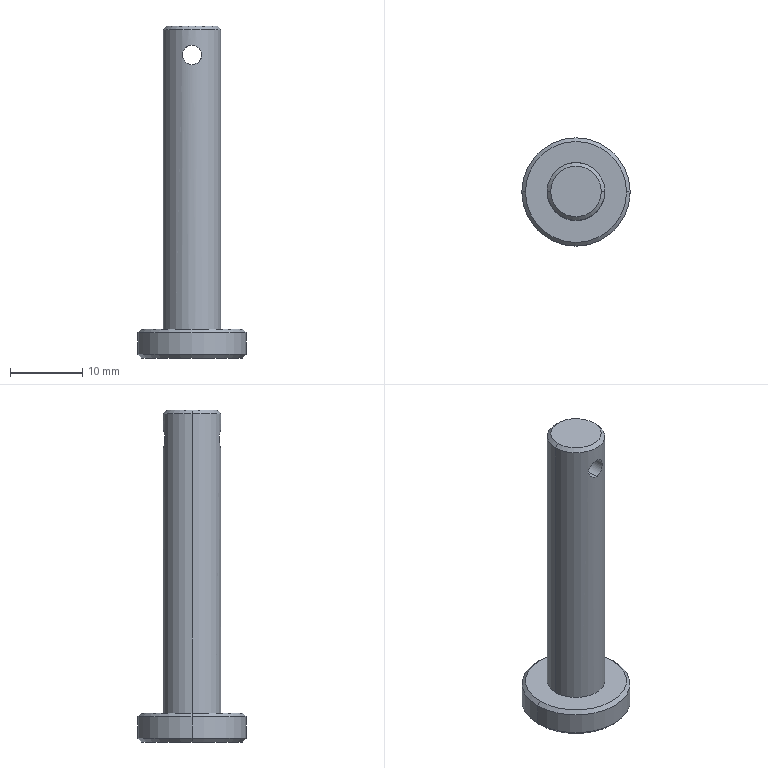Part | SolidWorks | features ICE 2, Chamfer 1, Extrusion 1 | 1 solid | 15 faces | box 15 x 15 x 46 mm | volume 2758 mm3 | cone 6 | cylinder 6 | plane 3 | commonest cylinder face diameters 2.7 x2 8 x2 15 x2
STEP:
#1=CARTESIAN_POINT('',(3.5,0.,42.));
#2=VERTEX_POINT('',#1);
#3=CARTESIAN_POINT('',(-3.5,0.,42.));
#4=VERTEX_POINT('',#3);
#5=CARTESIAN_POINT('',(0.,0.,42.));
#6=DIRECTION('',(0.,0.,1.));
#7=DIRECTION('',(1.,0.,0.));
#8=AXIS2_PLACEMENT_3D('',#5,#6,#7);
#9=CIRCLE('',#8,3.5);
#10=EDGE_CURVE('',#2,#4,#9,.T.);
#11=ORIENTED_EDGE('',*,*,#10,.F.);
#12=CARTESIAN_POINT('',(4.,0.,41.5));
#13=VERTEX_POINT('',#12);
#14=CARTESIAN_POINT('',(3.5,0.,42.));
#15=DIRECTION('',(0.7071,0.,-0.7071));
#16=VECTOR('',#15,1000.);
#17=LINE('',#14,#16);
#18=EDGE_CURVE('',#2,#13,#17,.T.);
#19=ORIENTED_EDGE('',*,*,#18,.T.);
#20=CARTESIAN_POINT('',(-4.,0.,41.5));
#21=VERTEX_POINT('',#20);
#22=CARTESIAN_POINT('',(0.,0.,41.5));
#23=DIRECTION('',(0.,0.,-1.));
#24=DIRECTION('',(1.,0.,0.));
#25=AXIS2_PLACEMENT_3D('',#22,#23,#24);
#26=CIRCLE('',#25,4.);
#27=EDGE_CURVE('',#21,#13,#26,.T.);
#28=ORIENTED_EDGE('',*,*,#27,.F.);
#29=CARTESIAN_POINT('',(-3.5,0.,42.));
#30=DIRECTION('',(-0.7071,0.,-0.7071));
#31=VECTOR('',#30,1000.);
#32=LINE('',#29,#31);
#33=EDGE_CURVE('',#4,#21,#32,.T.);
#34=ORIENTED_EDGE('',*,*,#33,.F.);
#35=EDGE_LOOP('',(#11,#19,#28,#34));
#36=FACE_OUTER_BOUND('',#35,.T.);
#37=CARTESIAN_POINT('',(0.,0.,42.));
#38=DIRECTION('',(0.,0.,-1.));
#39=DIRECTION('',(-1.,0.,0.));
#40=AXIS2_PLACEMENT_3D('',#37,#38,#39);
#41=CONICAL_SURFACE('',#40,3.5,0.7854);
#42=ADVANCED_FACE('',(#36),#41,.T.);
#43=CARTESIAN_POINT('',(7.,0.,0.));
#44=VERTEX_POINT('',#43);
#45=CARTESIAN_POINT('',(-7.,0.,0.));
#46=VERTEX_POINT('',#45);
#47=CARTESIAN_POINT('',(0.,0.,0.));
#48=DIRECTION('',(0.,0.,1.));
#49=DIRECTION('',(-1.,0.,0.));
#50=AXIS2_PLACEMENT_3D('',#47,#48,#49);
#51=CIRCLE('',#50,7.);
#52=EDGE_CURVE('',#44,#46,#51,.T.);
#53=ORIENTED_EDGE('',*,*,#52,.F.);
#54=CARTESIAN_POINT('',(7.5,0.,-0.5));
#55=VERTEX_POINT('',#54);
#56=CARTESIAN_POINT('',(7.5,0.,-0.5));
#57=DIRECTION('',(0.7071,0.,-0.7071));
#58=VECTOR('',#57,1000.);
#59=LINE('',#56,#58);
#60=EDGE_CURVE('',#44,#55,#59,.T.);
#61=ORIENTED_EDGE('',*,*,#60,.T.);
#62=CARTESIAN_POINT('',(-7.5,0.,-0.5));
#63=VERTEX_POINT('',#62);
#64=CARTESIAN_POINT('',(0.,0.,-0.5));
#65=DIRECTION('',(0.,0.,-1.));
#66=DIRECTION('',(-1.,0.,0.));
#67=AXIS2_PLACEMENT_3D('',#64,#65,#66);
#68=CIRCLE('',#67,7.5);
#69=EDGE_CURVE('',#63,#55,#68,.T.);
#70=ORIENTED_EDGE('',*,*,#69,.F.);
#71=CARTESIAN_POINT('',(-7.5,0.,-0.5));
#72=DIRECTION('',(-0.7071,0.,-0.7071));
#73=VECTOR('',#72,1000.);
#74=LINE('',#71,#73);
#75=EDGE_CURVE('',#46,#63,#74,.T.);
#76=ORIENTED_EDGE('',*,*,#75,.F.);
#77=EDGE_LOOP('',(#53,#61,#70,#76));
#78=FACE_OUTER_BOUND('',#77,.T.);
#79=CARTESIAN_POINT('',(0.,0.,-0.5));
#80=DIRECTION('',(0.,0.,-1.));
#81=DIRECTION('',(-1.,0.,0.));
#82=AXIS2_PLACEMENT_3D('',#79,#80,#81);
#83=CONICAL_SURFACE('',#82,7.5,0.7854);
#84=ADVANCED_FACE('',(#78),#83,.T.);
#85=CARTESIAN_POINT('',(-7.,0.,-4.));
#86=VERTEX_POINT('',#85);
#87=CARTESIAN_POINT('',(7.,0.,-4.));
#88=VERTEX_POINT('',#87);
#89=CARTESIAN_POINT('',(0.,0.,-4.));
#90=DIRECTION('',(0.,0.,-1.));
#91=DIRECTION('',(-1.,0.,0.));
#92=AXIS2_PLACEMENT_3D('',#89,#90,#91);
#93=CIRCLE('',#92,7.);
#94=EDGE_CURVE('',#86,#88,#93,.T.);
#95=ORIENTED_EDGE('',*,*,#94,.F.);
#96=CARTESIAN_POINT('',(-7.5,0.,-3.5));
#97=VERTEX_POINT('',#96);
#98=CARTESIAN_POINT('',(-7.,0.,-4.));
#99=DIRECTION('',(-0.7071,0.,0.7071));
#100=VECTOR('',#99,1000.);
#101=LINE('',#98,#100);
#102=EDGE_CURVE('',#86,#97,#101,.T.);
#103=ORIENTED_EDGE('',*,*,#102,.T.);
#104=CARTESIAN_POINT('',(7.5,0.,-3.5));
#105=VERTEX_POINT('',#104);
#106=CARTESIAN_POINT('',(0.,0.,-3.5));
#107=DIRECTION('',(0.,0.,1.));
#108=DIRECTION('',(-1.,0.,0.));
#109=AXIS2_PLACEMENT_3D('',#106,#107,#108);
#110=CIRCLE('',#109,7.5);
#111=EDGE_CURVE('',#105,#97,#110,.T.);
#112=ORIENTED_EDGE('',*,*,#111,.F.);
#113=CARTESIAN_POINT('',(7.,0.,-4.));
#114=DIRECTION('',(0.7071,0.,0.7071));
#115=VECTOR('',#114,1000.);
#116=LINE('',#113,#115);
#117=EDGE_CURVE('',#88,#105,#116,.T.);
#118=ORIENTED_EDGE('',*,*,#117,.F.);
#119=EDGE_LOOP('',(#95,#103,#112,#118));
#120=FACE_OUTER_BOUND('',#119,.T.);
#121=CARTESIAN_POINT('',(0.,0.,-4.));
#122=DIRECTION('',(0.,0.,1.));
#123=DIRECTION('',(1.,0.,0.));
#124=AXIS2_PLACEMENT_3D('',#121,#122,#123);
#125=CONICAL_SURFACE('',#124,7.,0.7854);
#126=ADVANCED_FACE('',(#120),#125,.T.);
#127=CARTESIAN_POINT('',(0.,-4.,36.65));
#128=VERTEX_POINT('',#127);
#129=CARTESIAN_POINT('',(0.,-4.,39.35));
#130=VERTEX_POINT('',#129);
#131=CARTESIAN_POINT('',(0.,-4.,36.65));
#132=CARTESIAN_POINT('',(-0.1771,-4.,36.65));
#133=CARTESIAN_POINT('',(-0.3558,-3.988,36.686));
#134=CARTESIAN_POINT('',(-0.6002,-3.956,36.788));
#135=CARTESIAN_POINT('',(-0.6792,-3.943,36.83));
#136=CARTESIAN_POINT('',(-0.8249,-3.915,36.928));
#137=CARTESIAN_POINT('',(-0.8925,-3.9,36.983));
#138=CARTESIAN_POINT('',(-1.079,-3.854,37.17));
#139=CARTESIAN_POINT('',(-1.178,-3.823,37.318));
#140=CARTESIAN_POINT('',(-1.281,-3.79,37.564));
#141=CARTESIAN_POINT('',(-1.306,-3.781,37.648));
#142=CARTESIAN_POINT('',(-1.341,-3.769,37.821));
#143=CARTESIAN_POINT('',(-1.35,-3.765,37.911));
#144=CARTESIAN_POINT('',(-1.35,-3.765,38.178));
#145=CARTESIAN_POINT('',(-1.314,-3.779,38.356));
#146=CARTESIAN_POINT('',(-1.179,-3.823,38.681));
#147=CARTESIAN_POINT('',(-1.078,-3.854,38.831));
#148=CARTESIAN_POINT('',(-0.8929,-3.9,39.016));
#149=CARTESIAN_POINT('',(-0.8239,-3.915,39.073));
#150=CARTESIAN_POINT('',(-0.6781,-3.943,39.171));
#151=CARTESIAN_POINT('',(-0.6009,-3.955,39.212));
#152=CARTESIAN_POINT('',(-0.4376,-3.977,39.28));
#153=CARTESIAN_POINT('',(-0.3516,-3.985,39.306));
#154=CARTESIAN_POINT('',(-0.1782,-3.997,39.341));
#155=CARTESIAN_POINT('',(-0.08989,-4.,39.35));
#156=CARTESIAN_POINT('',(0.,-4.,39.35));
#157=B_SPLINE_CURVE_WITH_KNOTS('',3,(#131,#132,#133,#134,#135,#136,#137,#138,#139,#140,#141,#142,#143,#144,#145,#146,#147,#148,#149,#150,#151,#152,#153,#154,#155,#156),.UNSPECIFIED.,.F.,.F.,(4,2,2,2,2,2,2,2,2,2,2,2,4),(0.004252,0.004784,0.005049,0.005315,0.005846,0.006112,0.006378,0.006909,0.007441,0.007706,0.007972,0.008238,0.008503),.UNSPECIFIED.);
#158=EDGE_CURVE('',#128,#130,#157,.T.);
#159=ORIENTED_EDGE('',*,*,#158,.F.);
#160=CARTESIAN_POINT('',(0.,4.,36.65));
#161=VERTEX_POINT('',#160);
#162=CARTESIAN_POINT('',(0.,-7.5,36.65));
#163=DIRECTION('',(0.,1.,0.));
#164=VECTOR('',#163,1000.);
#165=LINE('',#162,#164);
#166=EDGE_CURVE('',#128,#161,#165,.T.);
#167=ORIENTED_EDGE('',*,*,#166,.T.);
#168=CARTESIAN_POINT('',(0.,4.,39.35));
#169=VERTEX_POINT('',#168);
#170=CARTESIAN_POINT('',(0.,4.,39.35));
#171=CARTESIAN_POINT('',(-0.08991,4.,39.35));
#172=CARTESIAN_POINT('',(-0.1782,3.997,39.341));
#173=CARTESIAN_POINT('',(-0.3517,3.985,39.306));
#174=CARTESIAN_POINT('',(-0.4378,3.977,39.28));
#175=CARTESIAN_POINT('',(-0.6826,3.945,39.178));
#176=CARTESIAN_POINT('',(-0.8315,3.915,39.078));
#177=CARTESIAN_POINT('',(-1.079,3.854,38.831));
#178=CARTESIAN_POINT('',(-1.179,3.823,38.681));
#179=CARTESIAN_POINT('',(-1.314,3.779,38.357));
#180=CARTESIAN_POINT('',(-1.35,3.765,38.178));
#181=CARTESIAN_POINT('',(-1.35,3.765,37.912));
#182=CARTESIAN_POINT('',(-1.341,3.769,37.822));
#183=CARTESIAN_POINT('',(-1.306,3.781,37.648));
#184=CARTESIAN_POINT('',(-1.281,3.79,37.563));
#185=CARTESIAN_POINT('',(-1.178,3.823,37.317));
#186=CARTESIAN_POINT('',(-1.078,3.854,37.169));
#187=CARTESIAN_POINT('',(-0.8921,3.9,36.983));
#188=CARTESIAN_POINT('',(-0.8246,3.915,36.928));
#189=CARTESIAN_POINT('',(-0.6788,3.943,36.83));
#190=CARTESIAN_POINT('',(-0.5998,3.956,36.787));
#191=CARTESIAN_POINT('',(-0.3559,3.988,36.686));
#192=CARTESIAN_POINT('',(-0.1771,4.,36.65));
#193=CARTESIAN_POINT('',(0.,4.,36.65));
#194=B_SPLINE_CURVE_WITH_KNOTS('',3,(#170,#171,#172,#173,#174,#175,#176,#177,#178,#179,#180,#181,#182,#183,#184,#185,#186,#187,#188,#189,#190,#191,#192,#193),.UNSPECIFIED.,.F.,.F.,(4,2,2,2,2,2,2,2,2,2,2,4),(0.,0.0002658,0.0005315,0.001063,0.001595,0.002126,0.002392,0.002658,0.003189,0.003455,0.003721,0.004252),.UNSPECIFIED.);
#195=EDGE_CURVE('',#169,#161,#194,.T.);
#196=ORIENTED_EDGE('',*,*,#195,.F.);
#197=CARTESIAN_POINT('',(0.,-7.5,39.35));
#198=DIRECTION('',(0.,1.,0.));
#199=VECTOR('',#198,1000.);
#200=LINE('',#197,#199);
#201=EDGE_CURVE('',#130,#169,#200,.T.);
#202=ORIENTED_EDGE('',*,*,#201,.F.);
#203=EDGE_LOOP('',(#159,#167,#196,#202));
#204=FACE_OUTER_BOUND('',#203,.T.);
#205=CARTESIAN_POINT('',(0.,-7.5,38.));
#206=DIRECTION('',(0.,1.,0.));
#207=DIRECTION('',(0.,0.,1.));
#208=AXIS2_PLACEMENT_3D('',#205,#206,#207);
#209=CYLINDRICAL_SURFACE('',#208,1.35);
#210=ADVANCED_FACE('',(#204),#209,.F.);
#211=ORIENTED_EDGE('',*,*,#111,.T.);
#212=CARTESIAN_POINT('',(-7.5,0.,-4.));
#213=DIRECTION('',(0.,0.,1.));
#214=VECTOR('',#213,1000.);
#215=LINE('',#212,#214);
#216=EDGE_CURVE('',#97,#63,#215,.T.);
#217=ORIENTED_EDGE('',*,*,#216,.T.);
#218=ORIENTED_EDGE('',*,*,#69,.T.);
#219=CARTESIAN_POINT('',(7.5,0.,-4.));
#220=DIRECTION('',(0.,0.,1.));
#221=VECTOR('',#220,1000.);
#222=LINE('',#219,#221);
#223=EDGE_CURVE('',#105,#55,#222,.T.);
#224=ORIENTED_EDGE('',*,*,#223,.F.);
#225=EDGE_LOOP('',(#211,#217,#218,#224));
#226=FACE_OUTER_BOUND('',#225,.T.);
#227=CARTESIAN_POINT('',(0.,0.,-4.));
#228=DIRECTION('',(0.,0.,1.));
#229=DIRECTION('',(1.,0.,0.));
#230=AXIS2_PLACEMENT_3D('',#227,#228,#229);
#231=CYLINDRICAL_SURFACE('',#230,7.5);
#232=ADVANCED_FACE('',(#226),#231,.T.);
#233=ORIENTED_EDGE('',*,*,#195,.T.);
#234=CARTESIAN_POINT('',(0.,4.,36.65));
#235=CARTESIAN_POINT('',(0.1771,4.,36.65));
#236=CARTESIAN_POINT('',(0.3558,3.988,36.686));
#237=CARTESIAN_POINT('',(0.6002,3.956,36.788));
#238=CARTESIAN_POINT('',(0.6792,3.943,36.83));
#239=CARTESIAN_POINT('',(0.8249,3.915,36.928));
#240=CARTESIAN_POINT('',(0.8925,3.9,36.983));
#241=CARTESIAN_POINT('',(1.079,3.854,37.17));
#242=CARTESIAN_POINT('',(1.178,3.823,37.318));
#243=CARTESIAN_POINT('',(1.281,3.79,37.564));
#244=CARTESIAN_POINT('',(1.306,3.781,37.648));
#245=CARTESIAN_POINT('',(1.341,3.769,37.821));
#246=CARTESIAN_POINT('',(1.35,3.765,37.911));
#247=CARTESIAN_POINT('',(1.35,3.765,38.178));
#248=CARTESIAN_POINT('',(1.314,3.779,38.356));
#249=CARTESIAN_POINT('',(1.179,3.823,38.681));
#250=CARTESIAN_POINT('',(1.078,3.854,38.831));
#251=CARTESIAN_POINT('',(0.8929,3.9,39.016));
#252=CARTESIAN_POINT('',(0.8239,3.915,39.073));
#253=CARTESIAN_POINT('',(0.6781,3.943,39.171));
#254=CARTESIAN_POINT('',(0.6009,3.955,39.212));
#255=CARTESIAN_POINT('',(0.4376,3.977,39.28));
#256=CARTESIAN_POINT('',(0.3516,3.985,39.306));
#257=CARTESIAN_POINT('',(0.1782,3.997,39.341));
#258=CARTESIAN_POINT('',(0.08989,4.,39.35));
#259=CARTESIAN_POINT('',(0.,4.,39.35));
#260=B_SPLINE_CURVE_WITH_KNOTS('',3,(#234,#235,#236,#237,#238,#239,#240,#241,#242,#243,#244,#245,#246,#247,#248,#249,#250,#251,#252,#253,#254,#255,#256,#257,#258,#259),.UNSPECIFIED.,.F.,.F.,(4,2,2,2,2,2,2,2,2,2,2,2,4),(0.004252,0.004784,0.005049,0.005315,0.005846,0.006112,0.006378,0.006909,0.007441,0.007706,0.007972,0.008238,0.008503),.UNSPECIFIED.);
#261=EDGE_CURVE('',#161,#169,#260,.T.);
#262=ORIENTED_EDGE('',*,*,#261,.T.);
#263=EDGE_LOOP('',(#233,#262));
#264=FACE_BOUND('',#263,.T.);
#265=ORIENTED_EDGE('',*,*,#27,.T.);
#266=CARTESIAN_POINT('',(4.,0.,0.));
#267=VERTEX_POINT('',#266);
#268=CARTESIAN_POINT('',(4.,0.,42.));
#269=DIRECTION('',(0.,0.,-1.));
#270=VECTOR('',#269,1000.);
#271=LINE('',#268,#270);
#272=EDGE_CURVE('',#13,#267,#271,.T.);
#273=ORIENTED_EDGE('',*,*,#272,.T.);
#274=CARTESIAN_POINT('',(-4.,0.,0.));
#275=VERTEX_POINT('',#274);
#276=CARTESIAN_POINT('',(0.,0.,0.));
#277=DIRECTION('',(0.,0.,1.));
#278=DIRECTION('',(1.,0.,0.));
#279=AXIS2_PLACEMENT_3D('',#276,#277,#278);
#280=CIRCLE('',#279,4.);
#281=EDGE_CURVE('',#267,#275,#280,.T.);
#282=ORIENTED_EDGE('',*,*,#281,.T.);
#283=CARTESIAN_POINT('',(-4.,0.,42.));
#284=DIRECTION('',(0.,0.,-1.));
#285=VECTOR('',#284,1000.);
#286=LINE('',#283,#285);
#287=EDGE_CURVE('',#21,#275,#286,.T.);
#288=ORIENTED_EDGE('',*,*,#287,.F.);
#289=EDGE_LOOP('',(#265,#273,#282,#288));
#290=FACE_OUTER_BOUND('',#289,.T.);
#291=CARTESIAN_POINT('',(0.,0.,42.));
#292=DIRECTION('',(0.,0.,-1.));
#293=DIRECTION('',(-1.,0.,0.));
#294=AXIS2_PLACEMENT_3D('',#291,#292,#293);
#295=CYLINDRICAL_SURFACE('',#294,4.);
#296=ADVANCED_FACE('',(#264,#290),#295,.T.);
#297=ORIENTED_EDGE('',*,*,#272,.F.);
#298=CARTESIAN_POINT('',(0.,0.,41.5));
#299=DIRECTION('',(0.,0.,-1.));
#300=DIRECTION('',(1.,0.,0.));
#301=AXIS2_PLACEMENT_3D('',#298,#299,#300);
#302=CIRCLE('',#301,4.);
#303=EDGE_CURVE('',#13,#21,#302,.T.);
#304=ORIENTED_EDGE('',*,*,#303,.T.);
#305=ORIENTED_EDGE('',*,*,#287,.T.);
#306=CARTESIAN_POINT('',(0.,0.,0.));
#307=DIRECTION('',(0.,0.,1.));
#308=DIRECTION('',(1.,0.,0.));
#309=AXIS2_PLACEMENT_3D('',#306,#307,#308);
#310=CIRCLE('',#309,4.);
#311=EDGE_CURVE('',#275,#267,#310,.T.);
#312=ORIENTED_EDGE('',*,*,#311,.T.);
#313=EDGE_LOOP('',(#297,#304,#305,#312));
#314=FACE_OUTER_BOUND('',#313,.T.);
#315=CARTESIAN_POINT('',(0.,-4.,39.35));
#316=CARTESIAN_POINT('',(0.08991,-4.,39.35));
#317=CARTESIAN_POINT('',(0.1782,-3.997,39.341));
#318=CARTESIAN_POINT('',(0.3517,-3.985,39.306));
#319=CARTESIAN_POINT('',(0.4378,-3.977,39.28));
#320=CARTESIAN_POINT('',(0.6826,-3.945,39.178));
#321=CARTESIAN_POINT('',(0.8315,-3.915,39.078));
#322=CARTESIAN_POINT('',(1.079,-3.854,38.831));
#323=CARTESIAN_POINT('',(1.179,-3.823,38.681));
#324=CARTESIAN_POINT('',(1.314,-3.779,38.357));
#325=CARTESIAN_POINT('',(1.35,-3.765,38.178));
#326=CARTESIAN_POINT('',(1.35,-3.765,37.912));
#327=CARTESIAN_POINT('',(1.341,-3.769,37.822));
#328=CARTESIAN_POINT('',(1.306,-3.781,37.648));
#329=CARTESIAN_POINT('',(1.281,-3.79,37.563));
#330=CARTESIAN_POINT('',(1.178,-3.823,37.317));
#331=CARTESIAN_POINT('',(1.078,-3.854,37.169));
#332=CARTESIAN_POINT('',(0.8921,-3.9,36.983));
#333=CARTESIAN_POINT('',(0.8246,-3.915,36.928));
#334=CARTESIAN_POINT('',(0.6788,-3.943,36.83));
#335=CARTESIAN_POINT('',(0.5998,-3.956,36.787));
#336=CARTESIAN_POINT('',(0.3559,-3.988,36.686));
#337=CARTESIAN_POINT('',(0.1771,-4.,36.65));
#338=CARTESIAN_POINT('',(0.,-4.,36.65));
#339=B_SPLINE_CURVE_WITH_KNOTS('',3,(#315,#316,#317,#318,#319,#320,#321,#322,#323,#324,#325,#326,#327,#328,#329,#330,#331,#332,#333,#334,#335,#336,#337,#338),.UNSPECIFIED.,.F.,.F.,(4,2,2,2,2,2,2,2,2,2,2,4),(0.,0.0002658,0.0005315,0.001063,0.001595,0.002126,0.002392,0.002658,0.003189,0.003455,0.003721,0.004252),.UNSPECIFIED.);
#340=EDGE_CURVE('',#130,#128,#339,.T.);
#341=ORIENTED_EDGE('',*,*,#340,.T.);
#342=ORIENTED_EDGE('',*,*,#158,.T.);
#343=EDGE_LOOP('',(#341,#342));
#344=FACE_BOUND('',#343,.T.);
#345=CARTESIAN_POINT('',(0.,0.,42.));
#346=DIRECTION('',(0.,0.,-1.));
#347=DIRECTION('',(-1.,0.,0.));
#348=AXIS2_PLACEMENT_3D('',#345,#346,#347);
#349=CYLINDRICAL_SURFACE('',#348,4.);
#350=ADVANCED_FACE('',(#314,#344),#349,.T.);
#351=CARTESIAN_POINT('',(0.,0.,42.));
#352=DIRECTION('',(0.,0.,1.));
#353=DIRECTION('',(1.,0.,0.));
#354=AXIS2_PLACEMENT_3D('',#351,#352,#353);
#355=CIRCLE('',#354,3.5);
#356=EDGE_CURVE('',#4,#2,#355,.T.);
#357=ORIENTED_EDGE('',*,*,#356,.T.);
#358=ORIENTED_EDGE('',*,*,#10,.T.);
#359=EDGE_LOOP('',(#357,#358));
#360=FACE_OUTER_BOUND('',#359,.T.);
#361=CARTESIAN_POINT('',(0.,0.,42.));
#362=DIRECTION('',(0.,0.,1.));
#363=DIRECTION('',(1.,0.,0.));
#364=AXIS2_PLACEMENT_3D('',#361,#362,#363);
#365=PLANE('',#364);
#366=ADVANCED_FACE('',(#360),#365,.T.);
#367=ORIENTED_EDGE('',*,*,#216,.F.);
#368=CARTESIAN_POINT('',(0.,0.,-3.5));
#369=DIRECTION('',(0.,0.,1.));
#370=DIRECTION('',(-1.,0.,0.));
#371=AXIS2_PLACEMENT_3D('',#368,#369,#370);
#372=CIRCLE('',#371,7.5);
#373=EDGE_CURVE('',#97,#105,#372,.T.);
#374=ORIENTED_EDGE('',*,*,#373,.T.);
#375=ORIENTED_EDGE('',*,*,#223,.T.);
#376=CARTESIAN_POINT('',(0.,0.,-0.5));
#377=DIRECTION('',(0.,0.,-1.));
#378=DIRECTION('',(-1.,0.,0.));
#379=AXIS2_PLACEMENT_3D('',#376,#377,#378);
#380=CIRCLE('',#379,7.5);
#381=EDGE_CURVE('',#55,#63,#380,.T.);
#382=ORIENTED_EDGE('',*,*,#381,.T.);
#383=EDGE_LOOP('',(#367,#374,#375,#382));
#384=FACE_OUTER_BOUND('',#383,.T.);
#385=CARTESIAN_POINT('',(0.,0.,-4.));
#386=DIRECTION('',(0.,0.,1.));
#387=DIRECTION('',(1.,0.,0.));
#388=AXIS2_PLACEMENT_3D('',#385,#386,#387);
#389=CYLINDRICAL_SURFACE('',#388,7.5);
#390=ADVANCED_FACE('',(#384),#389,.T.);
#391=CARTESIAN_POINT('',(0.,0.,-4.));
#392=DIRECTION('',(0.,0.,-1.));
#393=DIRECTION('',(-1.,0.,0.));
#394=AXIS2_PLACEMENT_3D('',#391,#392,#393);
#395=CIRCLE('',#394,7.);
#396=EDGE_CURVE('',#88,#86,#395,.T.);
#397=ORIENTED_EDGE('',*,*,#396,.T.);
#398=ORIENTED_EDGE('',*,*,#94,.T.);
#399=EDGE_LOOP('',(#397,#398));
#400=FACE_OUTER_BOUND('',#399,.T.);
#401=CARTESIAN_POINT('',(0.,0.,-4.));
#402=DIRECTION('',(0.,0.,-1.));
#403=DIRECTION('',(-1.,0.,0.));
#404=AXIS2_PLACEMENT_3D('',#401,#402,#403);
#405=PLANE('',#404);
#406=ADVANCED_FACE('',(#400),#405,.T.);
#407=CARTESIAN_POINT('',(0.,0.,0.));
#408=DIRECTION('',(0.,0.,1.));
#409=DIRECTION('',(-1.,0.,0.));
#410=AXIS2_PLACEMENT_3D('',#407,#408,#409);
#411=CIRCLE('',#410,7.);
#412=EDGE_CURVE('',#46,#44,#411,.T.);
#413=ORIENTED_EDGE('',*,*,#412,.T.);
#414=ORIENTED_EDGE('',*,*,#52,.T.);
#415=EDGE_LOOP('',(#413,#414));
#416=FACE_OUTER_BOUND('',#415,.T.);
#417=ORIENTED_EDGE('',*,*,#311,.F.);
#418=ORIENTED_EDGE('',*,*,#281,.F.);
#419=EDGE_LOOP('',(#417,#418));
#420=FACE_BOUND('',#419,.T.);
#421=CARTESIAN_POINT('',(0.,0.,0.));
#422=DIRECTION('',(0.,0.,-1.));
#423=DIRECTION('',(-1.,0.,0.));
#424=AXIS2_PLACEMENT_3D('',#421,#422,#423);
#425=PLANE('',#424);
#426=ADVANCED_FACE('',(#416,#420),#425,.F.);
#427=ORIENTED_EDGE('',*,*,#166,.F.);
#428=ORIENTED_EDGE('',*,*,#340,.F.);
#429=ORIENTED_EDGE('',*,*,#201,.T.);
#430=ORIENTED_EDGE('',*,*,#261,.F.);
#431=EDGE_LOOP('',(#427,#428,#429,#430));
#432=FACE_OUTER_BOUND('',#431,.T.);
#433=CARTESIAN_POINT('',(0.,-7.5,38.));
#434=DIRECTION('',(0.,1.,0.));
#435=DIRECTION('',(0.,0.,1.));
#436=AXIS2_PLACEMENT_3D('',#433,#434,#435);
#437=CYLINDRICAL_SURFACE('',#436,1.35);
#438=ADVANCED_FACE('',(#432),#437,.F.);
#439=ORIENTED_EDGE('',*,*,#102,.F.);
#440=ORIENTED_EDGE('',*,*,#396,.F.);
#441=ORIENTED_EDGE('',*,*,#117,.T.);
#442=ORIENTED_EDGE('',*,*,#373,.F.);
#443=EDGE_LOOP('',(#439,#440,#441,#442));
#444=FACE_OUTER_BOUND('',#443,.T.);
#445=CARTESIAN_POINT('',(0.,0.,-4.));
#446=DIRECTION('',(0.,0.,1.));
#447=DIRECTION('',(1.,0.,0.));
#448=AXIS2_PLACEMENT_3D('',#445,#446,#447);
#449=CONICAL_SURFACE('',#448,7.,0.7854);
#450=ADVANCED_FACE('',(#444),#449,.T.);
#451=ORIENTED_EDGE('',*,*,#60,.F.);
#452=ORIENTED_EDGE('',*,*,#412,.F.);
#453=ORIENTED_EDGE('',*,*,#75,.T.);
#454=ORIENTED_EDGE('',*,*,#381,.F.);
#455=EDGE_LOOP('',(#451,#452,#453,#454));
#456=FACE_OUTER_BOUND('',#455,.T.);
#457=CARTESIAN_POINT('',(0.,0.,-0.5));
#458=DIRECTION('',(0.,0.,-1.));
#459=DIRECTION('',(-1.,0.,0.));
#460=AXIS2_PLACEMENT_3D('',#457,#458,#459);
#461=CONICAL_SURFACE('',#460,7.5,0.7854);
#462=ADVANCED_FACE('',(#456),#461,.T.);
#463=ORIENTED_EDGE('',*,*,#18,.F.);
#464=ORIENTED_EDGE('',*,*,#356,.F.);
#465=ORIENTED_EDGE('',*,*,#33,.T.);
#466=ORIENTED_EDGE('',*,*,#303,.F.);
#467=EDGE_LOOP('',(#463,#464,#465,#466));
#468=FACE_OUTER_BOUND('',#467,.T.);
#469=CARTESIAN_POINT('',(0.,0.,42.));
#470=DIRECTION('',(0.,0.,-1.));
#471=DIRECTION('',(-1.,0.,0.));
#472=AXIS2_PLACEMENT_3D('',#469,#470,#471);
#473=CONICAL_SURFACE('',#472,3.5,0.7854);
#474=ADVANCED_FACE('',(#468),#473,.T.);
#475=CLOSED_SHELL('',(#42,#84,#126,#210,#232,#296,#350,#366,#390,#406,#426,#438,#450,#462,#474));
#476=MANIFOLD_SOLID_BREP('',#475);
#477=CARTESIAN_POINT('',(0.,0.,0.));
#478=DIRECTION('',(0.,0.,1.));
#479=DIRECTION('',(1.,0.,0.));
#480=AXIS2_PLACEMENT_3D('',#477,#478,#479);
#481=(LENGTH_UNIT()NAMED_UNIT(*)SI_UNIT(.MILLI.,.METRE.));
#482=UNCERTAINTY_MEASURE_WITH_UNIT(LENGTH_MEASURE(0.00001),#481,'','');
#483=(NAMED_UNIT(*)PLANE_ANGLE_UNIT()SI_UNIT($,.RADIAN.));
#484=(NAMED_UNIT(*)SI_UNIT($,.STERADIAN.)SOLID_ANGLE_UNIT());
#485=(GEOMETRIC_REPRESENTATION_CONTEXT(3)GLOBAL_UNCERTAINTY_ASSIGNED_CONTEXT((#482))GLOBAL_UNIT_ASSIGNED_CONTEXT((#481,#483,#484))REPRESENTATION_CONTEXT('',''));
#486=ADVANCED_BREP_SHAPE_REPRESENTATION('',(#476,#480),#485);